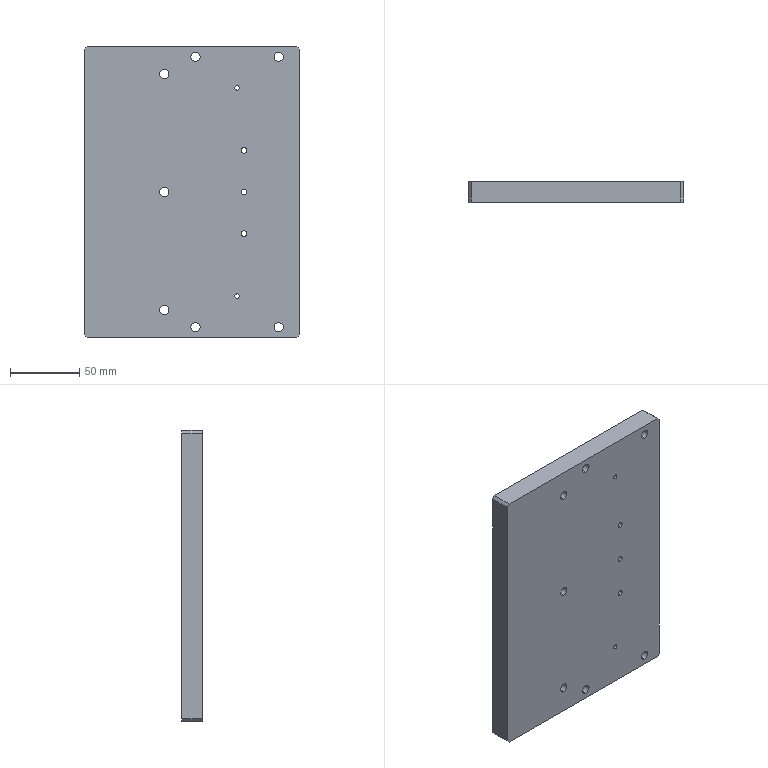Part | SolidWorks | features BaseBody 1 | 1 solid | 87 faces | box 155 x 15 x 210 mm | volume 479442 mm3 | cylinder 54 | plane 17 | cone 16 | commonest cylinder face diameters 3.3 x20 6.6 x14 11 x14 4.2 x6